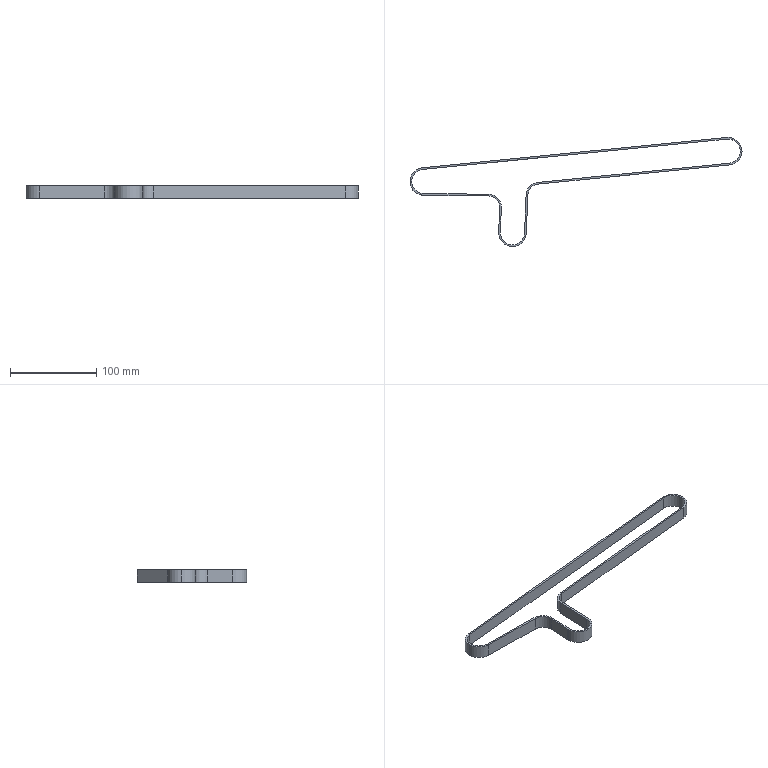Part | STEP file | HTBN918S3M-150 | 1 solid | 26 faces | box 383.9 x 126.27 x 15 mm | volume 27185 mm3 | cylinder 14 | plane 12 | commonest cylinder face diameters 27.9 x5 31.9 x5 25.8 x2 29.8 x2
STEP:
#1=CARTESIAN_POINT('',(-216.674,53.918,15.));
#2=VERTEX_POINT('',#1);
#3=CARTESIAN_POINT('',(-229.244,40.037,15.));
#4=VERTEX_POINT('',#3);
#5=CARTESIAN_POINT('',(-215.294,40.037,15.));
#6=DIRECTION('',(0.,0.,1.));
#7=DIRECTION('',(1.,0.,0.));
#8=AXIS2_PLACEMENT_3D('',#5,#6,#7);
#9=CIRCLE('',#8,13.95);
#10=EDGE_CURVE('',#2,#4,#9,.T.);
#11=ORIENTED_EDGE('',*,*,#10,.T.);
#12=CARTESIAN_POINT('',(-229.244,40.037,0.));
#13=VERTEX_POINT('',#12);
#14=CARTESIAN_POINT('',(-229.244,40.037,15.));
#15=DIRECTION('',(0.,0.,-1.));
#16=VECTOR('',#15,1000.);
#17=LINE('',#14,#16);
#18=EDGE_CURVE('',#4,#13,#17,.T.);
#19=ORIENTED_EDGE('',*,*,#18,.T.);
#20=CARTESIAN_POINT('',(-216.674,53.918,0.));
#21=VERTEX_POINT('',#20);
#22=CARTESIAN_POINT('',(-215.294,40.037,0.));
#23=DIRECTION('',(0.,0.,1.));
#24=DIRECTION('',(1.,0.,0.));
#25=AXIS2_PLACEMENT_3D('',#22,#23,#24);
#26=CIRCLE('',#25,13.95);
#27=EDGE_CURVE('',#21,#13,#26,.T.);
#28=ORIENTED_EDGE('',*,*,#27,.F.);
#29=CARTESIAN_POINT('',(-216.674,53.918,15.));
#30=DIRECTION('',(0.,0.,-1.));
#31=VECTOR('',#30,1000.);
#32=LINE('',#29,#31);
#33=EDGE_CURVE('',#2,#21,#32,.T.);
#34=ORIENTED_EDGE('',*,*,#33,.F.);
#35=EDGE_LOOP('',(#11,#19,#28,#34));
#36=FACE_OUTER_BOUND('',#35,.T.);
#37=CARTESIAN_POINT('',(-215.294,40.037,15.));
#38=DIRECTION('',(0.,0.,-1.));
#39=DIRECTION('',(-1.,0.,0.));
#40=AXIS2_PLACEMENT_3D('',#37,#38,#39);
#41=CYLINDRICAL_SURFACE('',#40,13.95);
#42=ADVANCED_FACE('',(#36),#41,.F.);
#43=CARTESIAN_POINT('',(-126.687,-18.819,15.));
#44=VERTEX_POINT('',#43);
#45=CARTESIAN_POINT('',(-126.697,-19.333,15.));
#46=VERTEX_POINT('',#45);
#47=CARTESIAN_POINT('',(-112.747,-19.333,15.));
#48=DIRECTION('',(0.,0.,1.));
#49=DIRECTION('',(1.,0.,0.));
#50=AXIS2_PLACEMENT_3D('',#47,#48,#49);
#51=CIRCLE('',#50,13.95);
#52=EDGE_CURVE('',#44,#46,#51,.T.);
#53=ORIENTED_EDGE('',*,*,#52,.T.);
#54=CARTESIAN_POINT('',(-126.697,-19.333,0.));
#55=VERTEX_POINT('',#54);
#56=CARTESIAN_POINT('',(-126.697,-19.333,15.));
#57=DIRECTION('',(0.,0.,-1.));
#58=VECTOR('',#57,1000.);
#59=LINE('',#56,#58);
#60=EDGE_CURVE('',#46,#55,#59,.T.);
#61=ORIENTED_EDGE('',*,*,#60,.T.);
#62=CARTESIAN_POINT('',(-126.687,-18.819,0.));
#63=VERTEX_POINT('',#62);
#64=CARTESIAN_POINT('',(-112.747,-19.333,0.));
#65=DIRECTION('',(0.,0.,1.));
#66=DIRECTION('',(1.,0.,0.));
#67=AXIS2_PLACEMENT_3D('',#64,#65,#66);
#68=CIRCLE('',#67,13.95);
#69=EDGE_CURVE('',#63,#55,#68,.T.);
#70=ORIENTED_EDGE('',*,*,#69,.F.);
#71=CARTESIAN_POINT('',(-126.687,-18.819,15.));
#72=DIRECTION('',(0.,0.,-1.));
#73=VECTOR('',#72,1000.);
#74=LINE('',#71,#73);
#75=EDGE_CURVE('',#44,#63,#74,.T.);
#76=ORIENTED_EDGE('',*,*,#75,.F.);
#77=EDGE_LOOP('',(#53,#61,#70,#76));
#78=FACE_OUTER_BOUND('',#77,.T.);
#79=CARTESIAN_POINT('',(-112.747,-19.333,15.));
#80=DIRECTION('',(0.,0.,-1.));
#81=DIRECTION('',(-1.,0.,0.));
#82=AXIS2_PLACEMENT_3D('',#79,#80,#81);
#83=CYLINDRICAL_SURFACE('',#82,13.95);
#84=ADVANCED_FACE('',(#78),#83,.F.);
#85=CARTESIAN_POINT('',(-128.697,-19.333,15.));
#86=VERTEX_POINT('',#85);
#87=CARTESIAN_POINT('',(-96.81,-19.979,15.));
#88=VERTEX_POINT('',#87);
#89=CARTESIAN_POINT('',(-112.747,-19.333,15.));
#90=DIRECTION('',(0.,0.,1.));
#91=DIRECTION('',(1.,0.,0.));
#92=AXIS2_PLACEMENT_3D('',#89,#90,#91);
#93=CIRCLE('',#92,15.95);
#94=EDGE_CURVE('',#86,#88,#93,.T.);
#95=ORIENTED_EDGE('',*,*,#94,.F.);
#96=CARTESIAN_POINT('',(-128.697,-19.333,0.));
#97=VERTEX_POINT('',#96);
#98=CARTESIAN_POINT('',(-128.697,-19.333,15.));
#99=DIRECTION('',(0.,0.,-1.));
#100=VECTOR('',#99,1000.);
#101=LINE('',#98,#100);
#102=EDGE_CURVE('',#86,#97,#101,.T.);
#103=ORIENTED_EDGE('',*,*,#102,.T.);
#104=CARTESIAN_POINT('',(-96.81,-19.979,0.));
#105=VERTEX_POINT('',#104);
#106=CARTESIAN_POINT('',(-112.747,-19.333,0.));
#107=DIRECTION('',(0.,0.,1.));
#108=DIRECTION('',(1.,0.,0.));
#109=AXIS2_PLACEMENT_3D('',#106,#107,#108);
#110=CIRCLE('',#109,15.95);
#111=EDGE_CURVE('',#97,#105,#110,.T.);
#112=ORIENTED_EDGE('',*,*,#111,.T.);
#113=CARTESIAN_POINT('',(-96.81,-19.979,15.));
#114=DIRECTION('',(0.,0.,-1.));
#115=VECTOR('',#114,1000.);
#116=LINE('',#113,#115);
#117=EDGE_CURVE('',#88,#105,#116,.T.);
#118=ORIENTED_EDGE('',*,*,#117,.F.);
#119=EDGE_LOOP('',(#95,#103,#112,#118));
#120=FACE_OUTER_BOUND('',#119,.T.);
#121=CARTESIAN_POINT('',(-112.747,-19.333,15.));
#122=DIRECTION('',(0.,0.,-1.));
#123=DIRECTION('',(-1.,0.,0.));
#124=AXIS2_PLACEMENT_3D('',#121,#122,#123);
#125=CYLINDRICAL_SURFACE('',#124,15.95);
#126=ADVANCED_FACE('',(#120),#125,.T.);
#127=CARTESIAN_POINT('',(-231.244,40.037,15.));
#128=VERTEX_POINT('',#127);
#129=CARTESIAN_POINT('',(-215.472,24.088,15.));
#130=VERTEX_POINT('',#129);
#131=CARTESIAN_POINT('',(-215.294,40.037,15.));
#132=DIRECTION('',(0.,0.,1.));
#133=DIRECTION('',(1.,0.,0.));
#134=AXIS2_PLACEMENT_3D('',#131,#132,#133);
#135=CIRCLE('',#134,15.95);
#136=EDGE_CURVE('',#128,#130,#135,.T.);
#137=ORIENTED_EDGE('',*,*,#136,.F.);
#138=CARTESIAN_POINT('',(-231.244,40.037,0.));
#139=VERTEX_POINT('',#138);
#140=CARTESIAN_POINT('',(-231.244,40.037,15.));
#141=DIRECTION('',(0.,0.,-1.));
#142=VECTOR('',#141,1000.);
#143=LINE('',#140,#142);
#144=EDGE_CURVE('',#128,#139,#143,.T.);
#145=ORIENTED_EDGE('',*,*,#144,.T.);
#146=CARTESIAN_POINT('',(-215.472,24.088,0.));
#147=VERTEX_POINT('',#146);
#148=CARTESIAN_POINT('',(-215.294,40.037,0.));
#149=DIRECTION('',(0.,0.,1.));
#150=DIRECTION('',(1.,0.,0.));
#151=AXIS2_PLACEMENT_3D('',#148,#149,#150);
#152=CIRCLE('',#151,15.95);
#153=EDGE_CURVE('',#139,#147,#152,.T.);
#154=ORIENTED_EDGE('',*,*,#153,.T.);
#155=CARTESIAN_POINT('',(-215.472,24.088,15.));
#156=DIRECTION('',(0.,0.,-1.));
#157=VECTOR('',#156,1000.);
#158=LINE('',#155,#157);
#159=EDGE_CURVE('',#130,#147,#158,.T.);
#160=ORIENTED_EDGE('',*,*,#159,.F.);
#161=EDGE_LOOP('',(#137,#145,#154,#160));
#162=FACE_OUTER_BOUND('',#161,.T.);
#163=CARTESIAN_POINT('',(-215.294,40.037,15.));
#164=DIRECTION('',(0.,0.,-1.));
#165=DIRECTION('',(-1.,0.,0.));
#166=AXIS2_PLACEMENT_3D('',#163,#164,#165);
#167=CYLINDRICAL_SURFACE('',#166,15.95);
#168=ADVANCED_FACE('',(#162),#167,.T.);
#169=CARTESIAN_POINT('',(-216.872,55.909,15.));
#170=VERTEX_POINT('',#169);
#171=CARTESIAN_POINT('',(-215.294,40.037,15.));
#172=DIRECTION('',(0.,0.,1.));
#173=DIRECTION('',(1.,0.,0.));
#174=AXIS2_PLACEMENT_3D('',#171,#172,#173);
#175=CIRCLE('',#174,15.95);
#176=EDGE_CURVE('',#170,#128,#175,.T.);
#177=ORIENTED_EDGE('',*,*,#176,.T.);
#178=ORIENTED_EDGE('',*,*,#136,.T.);
#179=CARTESIAN_POINT('',(-140.379,23.251,15.));
#180=VERTEX_POINT('',#179);
#181=CARTESIAN_POINT('',(-215.472,24.088,15.));
#182=DIRECTION('',(0.9999,-0.01115,0.));
#183=VECTOR('',#182,1000.);
#184=LINE('',#181,#183);
#185=EDGE_CURVE('',#130,#180,#184,.T.);
#186=ORIENTED_EDGE('',*,*,#185,.T.);
#187=CARTESIAN_POINT('',(-127.631,9.876,15.));
#188=VERTEX_POINT('',#187);
#189=CARTESIAN_POINT('',(-140.522,10.351,15.));
#190=DIRECTION('',(0.,0.,-1.));
#191=DIRECTION('',(1.,0.,0.));
#192=AXIS2_PLACEMENT_3D('',#189,#190,#191);
#193=CIRCLE('',#192,12.9);
#194=EDGE_CURVE('',#180,#188,#193,.T.);
#195=ORIENTED_EDGE('',*,*,#194,.T.);
#196=CARTESIAN_POINT('',(-128.686,-18.745,15.));
#197=VERTEX_POINT('',#196);
#198=CARTESIAN_POINT('',(-127.631,9.876,15.));
#199=DIRECTION('',(-0.03683,-0.9993,0.));
#200=VECTOR('',#199,1000.);
#201=LINE('',#198,#200);
#202=EDGE_CURVE('',#188,#197,#201,.T.);
#203=ORIENTED_EDGE('',*,*,#202,.T.);
#204=CARTESIAN_POINT('',(-112.747,-19.333,15.));
#205=DIRECTION('',(0.,0.,1.));
#206=DIRECTION('',(1.,0.,0.));
#207=AXIS2_PLACEMENT_3D('',#204,#205,#206);
#208=CIRCLE('',#207,15.95);
#209=EDGE_CURVE('',#197,#86,#208,.T.);
#210=ORIENTED_EDGE('',*,*,#209,.T.);
#211=ORIENTED_EDGE('',*,*,#94,.T.);
#212=CARTESIAN_POINT('',(-95.002,24.597,15.));
#213=VERTEX_POINT('',#212);
#214=CARTESIAN_POINT('',(-95.002,24.597,15.));
#215=DIRECTION('',(0.04052,0.9992,0.));
#216=VECTOR('',#215,1000.);
#217=LINE('',#214,#216);
#218=EDGE_CURVE('',#88,#213,#217,.T.);
#219=ORIENTED_EDGE('',*,*,#218,.T.);
#220=CARTESIAN_POINT('',(-83.401,36.91,15.));
#221=VERTEX_POINT('',#220);
#222=CARTESIAN_POINT('',(-82.113,24.074,15.));
#223=DIRECTION('',(0.,0.,-1.));
#224=DIRECTION('',(1.,0.,0.));
#225=AXIS2_PLACEMENT_3D('',#222,#223,#224);
#226=CIRCLE('',#225,12.9);
#227=EDGE_CURVE('',#213,#221,#226,.T.);
#228=ORIENTED_EDGE('',*,*,#227,.T.);
#229=CARTESIAN_POINT('',(138.299,59.167,15.));
#230=VERTEX_POINT('',#229);
#231=CARTESIAN_POINT('',(-83.401,36.91,15.));
#232=DIRECTION('',(0.995,0.09989,0.));
#233=VECTOR('',#232,1000.);
#234=LINE('',#231,#233);
#235=EDGE_CURVE('',#221,#230,#234,.T.);
#236=ORIENTED_EDGE('',*,*,#235,.T.);
#237=CARTESIAN_POINT('',(135.128,90.909,15.));
#238=VERTEX_POINT('',#237);
#239=CARTESIAN_POINT('',(136.706,75.037,15.));
#240=DIRECTION('',(0.,0.,1.));
#241=DIRECTION('',(1.,0.,0.));
#242=AXIS2_PLACEMENT_3D('',#239,#240,#241);
#243=CIRCLE('',#242,15.95);
#244=EDGE_CURVE('',#230,#238,#243,.T.);
#245=ORIENTED_EDGE('',*,*,#244,.T.);
#246=CARTESIAN_POINT('',(-216.872,55.909,15.));
#247=DIRECTION('',(-0.9951,-0.09894,0.));
#248=VECTOR('',#247,1000.);
#249=LINE('',#246,#248);
#250=EDGE_CURVE('',#238,#170,#249,.T.);
#251=ORIENTED_EDGE('',*,*,#250,.T.);
#252=EDGE_LOOP('',(#177,#178,#186,#195,#203,#210,#211,#219,#228,#236,#245,#251));
#253=FACE_OUTER_BOUND('',#252,.T.);
#254=CARTESIAN_POINT('',(-125.633,9.803,15.));
#255=VERTEX_POINT('',#254);
#256=CARTESIAN_POINT('',(-125.633,9.803,15.));
#257=DIRECTION('',(-0.03683,-0.9993,0.));
#258=VECTOR('',#257,1000.);
#259=LINE('',#256,#258);
#260=EDGE_CURVE('',#255,#44,#259,.T.);
#261=ORIENTED_EDGE('',*,*,#260,.F.);
#262=CARTESIAN_POINT('',(-140.356,25.25,15.));
#263=VERTEX_POINT('',#262);
#264=CARTESIAN_POINT('',(-140.522,10.351,15.));
#265=DIRECTION('',(0.,0.,-1.));
#266=DIRECTION('',(1.,0.,0.));
#267=AXIS2_PLACEMENT_3D('',#264,#265,#266);
#268=CIRCLE('',#267,14.9);
#269=EDGE_CURVE('',#263,#255,#268,.T.);
#270=ORIENTED_EDGE('',*,*,#269,.F.);
#271=CARTESIAN_POINT('',(-215.449,26.088,15.));
#272=VERTEX_POINT('',#271);
#273=CARTESIAN_POINT('',(-215.449,26.088,15.));
#274=DIRECTION('',(0.9999,-0.01115,0.));
#275=VECTOR('',#274,1000.);
#276=LINE('',#273,#275);
#277=EDGE_CURVE('',#272,#263,#276,.T.);
#278=ORIENTED_EDGE('',*,*,#277,.F.);
#279=CARTESIAN_POINT('',(-215.294,40.037,15.));
#280=DIRECTION('',(0.,0.,1.));
#281=DIRECTION('',(1.,0.,0.));
#282=AXIS2_PLACEMENT_3D('',#279,#280,#281);
#283=CIRCLE('',#282,13.95);
#284=EDGE_CURVE('',#4,#272,#283,.T.);
#285=ORIENTED_EDGE('',*,*,#284,.F.);
#286=ORIENTED_EDGE('',*,*,#10,.F.);
#287=CARTESIAN_POINT('',(135.326,88.918,15.));
#288=VERTEX_POINT('',#287);
#289=CARTESIAN_POINT('',(-216.674,53.918,15.));
#290=DIRECTION('',(-0.9951,-0.09894,0.));
#291=VECTOR('',#290,1000.);
#292=LINE('',#289,#291);
#293=EDGE_CURVE('',#288,#2,#292,.T.);
#294=ORIENTED_EDGE('',*,*,#293,.F.);
#295=CARTESIAN_POINT('',(138.1,61.157,15.));
#296=VERTEX_POINT('',#295);
#297=CARTESIAN_POINT('',(136.706,75.037,15.));
#298=DIRECTION('',(0.,0.,1.));
#299=DIRECTION('',(1.,0.,0.));
#300=AXIS2_PLACEMENT_3D('',#297,#298,#299);
#301=CIRCLE('',#300,13.95);
#302=EDGE_CURVE('',#296,#288,#301,.T.);
#303=ORIENTED_EDGE('',*,*,#302,.F.);
#304=CARTESIAN_POINT('',(-83.601,38.9,15.));
#305=VERTEX_POINT('',#304);
#306=CARTESIAN_POINT('',(-83.601,38.9,15.));
#307=DIRECTION('',(0.995,0.09989,0.));
#308=VECTOR('',#307,1000.);
#309=LINE('',#306,#308);
#310=EDGE_CURVE('',#305,#296,#309,.T.);
#311=ORIENTED_EDGE('',*,*,#310,.F.);
#312=CARTESIAN_POINT('',(-97.001,24.678,15.));
#313=VERTEX_POINT('',#312);
#314=CARTESIAN_POINT('',(-82.113,24.074,15.));
#315=DIRECTION('',(0.,0.,-1.));
#316=DIRECTION('',(1.,0.,0.));
#317=AXIS2_PLACEMENT_3D('',#314,#315,#316);
#318=CIRCLE('',#317,14.9);
#319=EDGE_CURVE('',#313,#305,#318,.T.);
#320=ORIENTED_EDGE('',*,*,#319,.F.);
#321=CARTESIAN_POINT('',(-98.808,-19.898,15.));
#322=VERTEX_POINT('',#321);
#323=CARTESIAN_POINT('',(-97.001,24.678,15.));
#324=DIRECTION('',(0.04052,0.9992,0.));
#325=VECTOR('',#324,1000.);
#326=LINE('',#323,#325);
#327=EDGE_CURVE('',#322,#313,#326,.T.);
#328=ORIENTED_EDGE('',*,*,#327,.F.);
#329=CARTESIAN_POINT('',(-112.747,-19.333,15.));
#330=DIRECTION('',(0.,0.,1.));
#331=DIRECTION('',(1.,0.,0.));
#332=AXIS2_PLACEMENT_3D('',#329,#330,#331);
#333=CIRCLE('',#332,13.95);
#334=EDGE_CURVE('',#46,#322,#333,.T.);
#335=ORIENTED_EDGE('',*,*,#334,.F.);
#336=ORIENTED_EDGE('',*,*,#52,.F.);
#337=EDGE_LOOP('',(#261,#270,#278,#285,#286,#294,#303,#311,#320,#328,#335,#336));
#338=FACE_BOUND('',#337,.T.);
#339=CARTESIAN_POINT('',(-215.294,40.037,15.));
#340=DIRECTION('',(0.,0.,1.));
#341=DIRECTION('',(1.,0.,0.));
#342=AXIS2_PLACEMENT_3D('',#339,#340,#341);
#343=PLANE('',#342);
#344=ADVANCED_FACE('',(#253,#338),#343,.T.);
#345=CARTESIAN_POINT('',(-216.872,55.909,0.));
#346=VERTEX_POINT('',#345);
#347=CARTESIAN_POINT('',(-215.294,40.037,0.));
#348=DIRECTION('',(0.,0.,1.));
#349=DIRECTION('',(1.,0.,0.));
#350=AXIS2_PLACEMENT_3D('',#347,#348,#349);
#351=CIRCLE('',#350,15.95);
#352=EDGE_CURVE('',#346,#139,#351,.T.);
#353=ORIENTED_EDGE('',*,*,#352,.F.);
#354=CARTESIAN_POINT('',(135.128,90.909,0.));
#355=VERTEX_POINT('',#354);
#356=CARTESIAN_POINT('',(-216.872,55.909,0.));
#357=DIRECTION('',(-0.9951,-0.09894,0.));
#358=VECTOR('',#357,1000.);
#359=LINE('',#356,#358);
#360=EDGE_CURVE('',#355,#346,#359,.T.);
#361=ORIENTED_EDGE('',*,*,#360,.F.);
#362=CARTESIAN_POINT('',(138.299,59.167,0.));
#363=VERTEX_POINT('',#362);
#364=CARTESIAN_POINT('',(136.706,75.037,0.));
#365=DIRECTION('',(0.,0.,1.));
#366=DIRECTION('',(1.,0.,0.));
#367=AXIS2_PLACEMENT_3D('',#364,#365,#366);
#368=CIRCLE('',#367,15.95);
#369=EDGE_CURVE('',#363,#355,#368,.T.);
#370=ORIENTED_EDGE('',*,*,#369,.F.);
#371=CARTESIAN_POINT('',(-83.401,36.91,0.));
#372=VERTEX_POINT('',#371);
#373=CARTESIAN_POINT('',(-83.401,36.91,0.));
#374=DIRECTION('',(0.995,0.09989,0.));
#375=VECTOR('',#374,1000.);
#376=LINE('',#373,#375);
#377=EDGE_CURVE('',#372,#363,#376,.T.);
#378=ORIENTED_EDGE('',*,*,#377,.F.);
#379=CARTESIAN_POINT('',(-95.002,24.597,0.));
#380=VERTEX_POINT('',#379);
#381=CARTESIAN_POINT('',(-82.113,24.074,0.));
#382=DIRECTION('',(0.,0.,-1.));
#383=DIRECTION('',(1.,0.,0.));
#384=AXIS2_PLACEMENT_3D('',#381,#382,#383);
#385=CIRCLE('',#384,12.9);
#386=EDGE_CURVE('',#380,#372,#385,.T.);
#387=ORIENTED_EDGE('',*,*,#386,.F.);
#388=CARTESIAN_POINT('',(-95.002,24.597,0.));
#389=DIRECTION('',(0.04052,0.9992,0.));
#390=VECTOR('',#389,1000.);
#391=LINE('',#388,#390);
#392=EDGE_CURVE('',#105,#380,#391,.T.);
#393=ORIENTED_EDGE('',*,*,#392,.F.);
#394=ORIENTED_EDGE('',*,*,#111,.F.);
#395=CARTESIAN_POINT('',(-128.686,-18.745,0.));
#396=VERTEX_POINT('',#395);
#397=CARTESIAN_POINT('',(-112.747,-19.333,0.));
#398=DIRECTION('',(0.,0.,1.));
#399=DIRECTION('',(1.,0.,0.));
#400=AXIS2_PLACEMENT_3D('',#397,#398,#399);
#401=CIRCLE('',#400,15.95);
#402=EDGE_CURVE('',#396,#97,#401,.T.);
#403=ORIENTED_EDGE('',*,*,#402,.F.);
#404=CARTESIAN_POINT('',(-127.631,9.876,0.));
#405=VERTEX_POINT('',#404);
#406=CARTESIAN_POINT('',(-127.631,9.876,0.));
#407=DIRECTION('',(-0.03683,-0.9993,0.));
#408=VECTOR('',#407,1000.);
#409=LINE('',#406,#408);
#410=EDGE_CURVE('',#405,#396,#409,.T.);
#411=ORIENTED_EDGE('',*,*,#410,.F.);
#412=CARTESIAN_POINT('',(-140.379,23.251,0.));
#413=VERTEX_POINT('',#412);
#414=CARTESIAN_POINT('',(-140.522,10.351,0.));
#415=DIRECTION('',(0.,0.,-1.));
#416=DIRECTION('',(1.,0.,0.));
#417=AXIS2_PLACEMENT_3D('',#414,#415,#416);
#418=CIRCLE('',#417,12.9);
#419=EDGE_CURVE('',#413,#405,#418,.T.);
#420=ORIENTED_EDGE('',*,*,#419,.F.);
#421=CARTESIAN_POINT('',(-215.472,24.088,0.));
#422=DIRECTION('',(0.9999,-0.01115,0.));
#423=VECTOR('',#422,1000.);
#424=LINE('',#421,#423);
#425=EDGE_CURVE('',#147,#413,#424,.T.);
#426=ORIENTED_EDGE('',*,*,#425,.F.);
#427=ORIENTED_EDGE('',*,*,#153,.F.);
#428=EDGE_LOOP('',(#353,#361,#370,#378,#387,#393,#394,#403,#411,#420,#426,#427));
#429=FACE_OUTER_BOUND('',#428,.T.);
#430=CARTESIAN_POINT('',(-140.356,25.25,0.));
#431=VERTEX_POINT('',#430);
#432=CARTESIAN_POINT('',(-125.633,9.803,0.));
#433=VERTEX_POINT('',#432);
#434=CARTESIAN_POINT('',(-140.522,10.351,0.));
#435=DIRECTION('',(0.,0.,-1.));
#436=DIRECTION('',(1.,0.,0.));
#437=AXIS2_PLACEMENT_3D('',#434,#435,#436);
#438=CIRCLE('',#437,14.9);
#439=EDGE_CURVE('',#431,#433,#438,.T.);
#440=ORIENTED_EDGE('',*,*,#439,.T.);
#441=CARTESIAN_POINT('',(-125.633,9.803,0.));
#442=DIRECTION('',(-0.03683,-0.9993,0.));
#443=VECTOR('',#442,1000.);
#444=LINE('',#441,#443);
#445=EDGE_CURVE('',#433,#63,#444,.T.);
#446=ORIENTED_EDGE('',*,*,#445,.T.);
#447=ORIENTED_EDGE('',*,*,#69,.T.);
#448=CARTESIAN_POINT('',(-98.808,-19.898,0.));
#449=VERTEX_POINT('',#448);
#450=CARTESIAN_POINT('',(-112.747,-19.333,0.));
#451=DIRECTION('',(0.,0.,1.));
#452=DIRECTION('',(1.,0.,0.));
#453=AXIS2_PLACEMENT_3D('',#450,#451,#452);
#454=CIRCLE('',#453,13.95);
#455=EDGE_CURVE('',#55,#449,#454,.T.);
#456=ORIENTED_EDGE('',*,*,#455,.T.);
#457=CARTESIAN_POINT('',(-97.001,24.678,0.));
#458=VERTEX_POINT('',#457);
#459=CARTESIAN_POINT('',(-97.001,24.678,0.));
#460=DIRECTION('',(0.04052,0.9992,0.));
#461=VECTOR('',#460,1000.);
#462=LINE('',#459,#461);
#463=EDGE_CURVE('',#449,#458,#462,.T.);
#464=ORIENTED_EDGE('',*,*,#463,.T.);
#465=CARTESIAN_POINT('',(-83.601,38.9,0.));
#466=VERTEX_POINT('',#465);
#467=CARTESIAN_POINT('',(-82.113,24.074,0.));
#468=DIRECTION('',(0.,0.,-1.));
#469=DIRECTION('',(1.,0.,0.));
#470=AXIS2_PLACEMENT_3D('',#467,#468,#469);
#471=CIRCLE('',#470,14.9);
#472=EDGE_CURVE('',#458,#466,#471,.T.);
#473=ORIENTED_EDGE('',*,*,#472,.T.);
#474=CARTESIAN_POINT('',(138.1,61.157,0.));
#475=VERTEX_POINT('',#474);
#476=CARTESIAN_POINT('',(-83.601,38.9,0.));
#477=DIRECTION('',(0.995,0.09989,0.));
#478=VECTOR('',#477,1000.);
#479=LINE('',#476,#478);
#480=EDGE_CURVE('',#466,#475,#479,.T.);
#481=ORIENTED_EDGE('',*,*,#480,.T.);
#482=CARTESIAN_POINT('',(135.326,88.918,0.));
#483=VERTEX_POINT('',#482);
#484=CARTESIAN_POINT('',(136.706,75.037,0.));
#485=DIRECTION('',(0.,0.,1.));
#486=DIRECTION('',(1.,0.,0.));
#487=AXIS2_PLACEMENT_3D('',#484,#485,#486);
#488=CIRCLE('',#487,13.95);
#489=EDGE_CURVE('',#475,#483,#488,.T.);
#490=ORIENTED_EDGE('',*,*,#489,.T.);
#491=CARTESIAN_POINT('',(-216.674,53.918,0.));
#492=DIRECTION('',(-0.9951,-0.09894,0.));
#493=VECTOR('',#492,1000.);
#494=LINE('',#491,#493);
#495=EDGE_CURVE('',#483,#21,#494,.T.);
#496=ORIENTED_EDGE('',*,*,#495,.T.);
#497=ORIENTED_EDGE('',*,*,#27,.T.);
#498=CARTESIAN_POINT('',(-215.449,26.088,0.));
#499=VERTEX_POINT('',#498);
#500=CARTESIAN_POINT('',(-215.294,40.037,0.));
#501=DIRECTION('',(0.,0.,1.));
#502=DIRECTION('',(1.,0.,0.));
#503=AXIS2_PLACEMENT_3D('',#500,#501,#502);
#504=CIRCLE('',#503,13.95);
#505=EDGE_CURVE('',#13,#499,#504,.T.);
#506=ORIENTED_EDGE('',*,*,#505,.T.);
#507=CARTESIAN_POINT('',(-215.449,26.088,0.));
#508=DIRECTION('',(0.9999,-0.01115,0.));
#509=VECTOR('',#508,1000.);
#510=LINE('',#507,#509);
#511=EDGE_CURVE('',#499,#431,#510,.T.);
#512=ORIENTED_EDGE('',*,*,#511,.T.);
#513=EDGE_LOOP('',(#440,#446,#447,#456,#464,#473,#481,#490,#496,#497,#506,#512));
#514=FACE_BOUND('',#513,.T.);
#515=CARTESIAN_POINT('',(-215.294,40.037,0.));
#516=DIRECTION('',(0.,0.,1.));
#517=DIRECTION('',(1.,0.,0.));
#518=AXIS2_PLACEMENT_3D('',#515,#516,#517);
#519=PLANE('',#518);
#520=ADVANCED_FACE('',(#429,#514),#519,.F.);
#521=ORIENTED_EDGE('',*,*,#144,.F.);
#522=ORIENTED_EDGE('',*,*,#176,.F.);
#523=CARTESIAN_POINT('',(-216.872,55.909,15.));
#524=DIRECTION('',(0.,0.,-1.));
#525=VECTOR('',#524,1000.);
#526=LINE('',#523,#525);
#527=EDGE_CURVE('',#170,#346,#526,.T.);
#528=ORIENTED_EDGE('',*,*,#527,.T.);
#529=ORIENTED_EDGE('',*,*,#352,.T.);
#530=EDGE_LOOP('',(#521,#522,#528,#529));
#531=FACE_OUTER_BOUND('',#530,.T.);
#532=CARTESIAN_POINT('',(-215.294,40.037,15.));
#533=DIRECTION('',(0.,0.,-1.));
#534=DIRECTION('',(-1.,0.,0.));
#535=AXIS2_PLACEMENT_3D('',#532,#533,#534);
#536=CYLINDRICAL_SURFACE('',#535,15.95);
#537=ADVANCED_FACE('',(#531),#536,.T.);
#538=ORIENTED_EDGE('',*,*,#425,.T.);
#539=CARTESIAN_POINT('',(-140.379,23.251,15.));
#540=DIRECTION('',(0.,0.,-1.));
#541=VECTOR('',#540,1000.);
#542=LINE('',#539,#541);
#543=EDGE_CURVE('',#180,#413,#542,.T.);
#544=ORIENTED_EDGE('',*,*,#543,.F.);
#545=ORIENTED_EDGE('',*,*,#185,.F.);
#546=ORIENTED_EDGE('',*,*,#159,.T.);
#547=EDGE_LOOP('',(#538,#544,#545,#546));
#548=FACE_OUTER_BOUND('',#547,.T.);
#549=CARTESIAN_POINT('',(-215.472,24.088,15.));
#550=DIRECTION('',(0.01115,0.9999,0.));
#551=DIRECTION('',(-0.9999,0.01115,0.));
#552=AXIS2_PLACEMENT_3D('',#549,#550,#551);
#553=PLANE('',#552);
#554=ADVANCED_FACE('',(#548),#553,.F.);
#555=ORIENTED_EDGE('',*,*,#419,.T.);
#556=CARTESIAN_POINT('',(-127.631,9.876,15.));
#557=DIRECTION('',(0.,0.,-1.));
#558=VECTOR('',#557,1000.);
#559=LINE('',#556,#558);
#560=EDGE_CURVE('',#188,#405,#559,.T.);
#561=ORIENTED_EDGE('',*,*,#560,.F.);
#562=ORIENTED_EDGE('',*,*,#194,.F.);
#563=ORIENTED_EDGE('',*,*,#543,.T.);
#564=EDGE_LOOP('',(#555,#561,#562,#563));
#565=FACE_OUTER_BOUND('',#564,.T.);
#566=CARTESIAN_POINT('',(-140.522,10.351,15.));
#567=DIRECTION('',(0.,0.,-1.));
#568=DIRECTION('',(-1.,0.,0.));
#569=AXIS2_PLACEMENT_3D('',#566,#567,#568);
#570=CYLINDRICAL_SURFACE('',#569,12.9);
#571=ADVANCED_FACE('',(#565),#570,.F.);
#572=ORIENTED_EDGE('',*,*,#410,.T.);
#573=CARTESIAN_POINT('',(-128.686,-18.745,15.));
#574=DIRECTION('',(0.,0.,-1.));
#575=VECTOR('',#574,1000.);
#576=LINE('',#573,#575);
#577=EDGE_CURVE('',#197,#396,#576,.T.);
#578=ORIENTED_EDGE('',*,*,#577,.F.);
#579=ORIENTED_EDGE('',*,*,#202,.F.);
#580=ORIENTED_EDGE('',*,*,#560,.T.);
#581=EDGE_LOOP('',(#572,#578,#579,#580));
#582=FACE_OUTER_BOUND('',#581,.T.);
#583=CARTESIAN_POINT('',(-127.631,9.876,15.));
#584=DIRECTION('',(0.9993,-0.03683,0.));
#585=DIRECTION('',(0.03683,0.9993,0.));
#586=AXIS2_PLACEMENT_3D('',#583,#584,#585);
#587=PLANE('',#586);
#588=ADVANCED_FACE('',(#582),#587,.F.);
#589=ORIENTED_EDGE('',*,*,#102,.F.);
#590=ORIENTED_EDGE('',*,*,#209,.F.);
#591=ORIENTED_EDGE('',*,*,#577,.T.);
#592=ORIENTED_EDGE('',*,*,#402,.T.);
#593=EDGE_LOOP('',(#589,#590,#591,#592));
#594=FACE_OUTER_BOUND('',#593,.T.);
#595=CARTESIAN_POINT('',(-112.747,-19.333,15.));
#596=DIRECTION('',(0.,0.,-1.));
#597=DIRECTION('',(-1.,0.,0.));
#598=AXIS2_PLACEMENT_3D('',#595,#596,#597);
#599=CYLINDRICAL_SURFACE('',#598,15.95);
#600=ADVANCED_FACE('',(#594),#599,.T.);
#601=ORIENTED_EDGE('',*,*,#392,.T.);
#602=CARTESIAN_POINT('',(-95.002,24.597,15.));
#603=DIRECTION('',(0.,0.,-1.));
#604=VECTOR('',#603,1000.);
#605=LINE('',#602,#604);
#606=EDGE_CURVE('',#213,#380,#605,.T.);
#607=ORIENTED_EDGE('',*,*,#606,.F.);
#608=ORIENTED_EDGE('',*,*,#218,.F.);
#609=ORIENTED_EDGE('',*,*,#117,.T.);
#610=EDGE_LOOP('',(#601,#607,#608,#609));
#611=FACE_OUTER_BOUND('',#610,.T.);
#612=CARTESIAN_POINT('',(-95.002,24.597,15.));
#613=DIRECTION('',(-0.9992,0.04052,0.));
#614=DIRECTION('',(-0.04052,-0.9992,0.));
#615=AXIS2_PLACEMENT_3D('',#612,#613,#614);
#616=PLANE('',#615);
#617=ADVANCED_FACE('',(#611),#616,.F.);
#618=ORIENTED_EDGE('',*,*,#386,.T.);
#619=CARTESIAN_POINT('',(-83.401,36.91,15.));
#620=DIRECTION('',(0.,0.,-1.));
#621=VECTOR('',#620,1000.);
#622=LINE('',#619,#621);
#623=EDGE_CURVE('',#221,#372,#622,.T.);
#624=ORIENTED_EDGE('',*,*,#623,.F.);
#625=ORIENTED_EDGE('',*,*,#227,.F.);
#626=ORIENTED_EDGE('',*,*,#606,.T.);
#627=EDGE_LOOP('',(#618,#624,#625,#626));
#628=FACE_OUTER_BOUND('',#627,.T.);
#629=CARTESIAN_POINT('',(-82.113,24.074,15.));
#630=DIRECTION('',(0.,0.,-1.));
#631=DIRECTION('',(-1.,0.,0.));
#632=AXIS2_PLACEMENT_3D('',#629,#630,#631);
#633=CYLINDRICAL_SURFACE('',#632,12.9);
#634=ADVANCED_FACE('',(#628),#633,.F.);
#635=ORIENTED_EDGE('',*,*,#377,.T.);
#636=CARTESIAN_POINT('',(138.299,59.167,15.));
#637=DIRECTION('',(0.,0.,-1.));
#638=VECTOR('',#637,1000.);
#639=LINE('',#636,#638);
#640=EDGE_CURVE('',#230,#363,#639,.T.);
#641=ORIENTED_EDGE('',*,*,#640,.F.);
#642=ORIENTED_EDGE('',*,*,#235,.F.);
#643=ORIENTED_EDGE('',*,*,#623,.T.);
#644=EDGE_LOOP('',(#635,#641,#642,#643));
#645=FACE_OUTER_BOUND('',#644,.T.);
#646=CARTESIAN_POINT('',(-83.401,36.91,15.));
#647=DIRECTION('',(-0.09989,0.995,0.));
#648=DIRECTION('',(-0.995,-0.09989,0.));
#649=AXIS2_PLACEMENT_3D('',#646,#647,#648);
#650=PLANE('',#649);
#651=ADVANCED_FACE('',(#645),#650,.F.);
#652=ORIENTED_EDGE('',*,*,#369,.T.);
#653=CARTESIAN_POINT('',(135.128,90.909,15.));
#654=DIRECTION('',(0.,0.,-1.));
#655=VECTOR('',#654,1000.);
#656=LINE('',#653,#655);
#657=EDGE_CURVE('',#238,#355,#656,.T.);
#658=ORIENTED_EDGE('',*,*,#657,.F.);
#659=ORIENTED_EDGE('',*,*,#244,.F.);
#660=ORIENTED_EDGE('',*,*,#640,.T.);
#661=EDGE_LOOP('',(#652,#658,#659,#660));
#662=FACE_OUTER_BOUND('',#661,.T.);
#663=CARTESIAN_POINT('',(136.706,75.037,15.));
#664=DIRECTION('',(0.,0.,-1.));
#665=DIRECTION('',(-1.,0.,0.));
#666=AXIS2_PLACEMENT_3D('',#663,#664,#665);
#667=CYLINDRICAL_SURFACE('',#666,15.95);
#668=ADVANCED_FACE('',(#662),#667,.T.);
#669=ORIENTED_EDGE('',*,*,#360,.T.);
#670=ORIENTED_EDGE('',*,*,#527,.F.);
#671=ORIENTED_EDGE('',*,*,#250,.F.);
#672=ORIENTED_EDGE('',*,*,#657,.T.);
#673=EDGE_LOOP('',(#669,#670,#671,#672));
#674=FACE_OUTER_BOUND('',#673,.T.);
#675=CARTESIAN_POINT('',(-216.872,55.909,15.));
#676=DIRECTION('',(0.09894,-0.9951,0.));
#677=DIRECTION('',(0.9951,0.09894,0.));
#678=AXIS2_PLACEMENT_3D('',#675,#676,#677);
#679=PLANE('',#678);
#680=ADVANCED_FACE('',(#674),#679,.F.);
#681=ORIENTED_EDGE('',*,*,#439,.F.);
#682=CARTESIAN_POINT('',(-140.356,25.25,15.));
#683=DIRECTION('',(0.,0.,-1.));
#684=VECTOR('',#683,1000.);
#685=LINE('',#682,#684);
#686=EDGE_CURVE('',#263,#431,#685,.T.);
#687=ORIENTED_EDGE('',*,*,#686,.F.);
#688=ORIENTED_EDGE('',*,*,#269,.T.);
#689=CARTESIAN_POINT('',(-125.633,9.803,15.));
#690=DIRECTION('',(0.,0.,-1.));
#691=VECTOR('',#690,1000.);
#692=LINE('',#689,#691);
#693=EDGE_CURVE('',#255,#433,#692,.T.);
#694=ORIENTED_EDGE('',*,*,#693,.T.);
#695=EDGE_LOOP('',(#681,#687,#688,#694));
#696=FACE_OUTER_BOUND('',#695,.T.);
#697=CARTESIAN_POINT('',(-140.522,10.351,15.));
#698=DIRECTION('',(0.,0.,-1.));
#699=DIRECTION('',(-1.,0.,0.));
#700=AXIS2_PLACEMENT_3D('',#697,#698,#699);
#701=CYLINDRICAL_SURFACE('',#700,14.9);
#702=ADVANCED_FACE('',(#696),#701,.T.);
#703=ORIENTED_EDGE('',*,*,#445,.F.);
#704=ORIENTED_EDGE('',*,*,#693,.F.);
#705=ORIENTED_EDGE('',*,*,#260,.T.);
#706=ORIENTED_EDGE('',*,*,#75,.T.);
#707=EDGE_LOOP('',(#703,#704,#705,#706));
#708=FACE_OUTER_BOUND('',#707,.T.);
#709=CARTESIAN_POINT('',(-125.633,9.803,15.));
#710=DIRECTION('',(0.9993,-0.03683,0.));
#711=DIRECTION('',(0.03683,0.9993,0.));
#712=AXIS2_PLACEMENT_3D('',#709,#710,#711);
#713=PLANE('',#712);
#714=ADVANCED_FACE('',(#708),#713,.T.);
#715=ORIENTED_EDGE('',*,*,#60,.F.);
#716=ORIENTED_EDGE('',*,*,#334,.T.);
#717=CARTESIAN_POINT('',(-98.808,-19.898,15.));
#718=DIRECTION('',(0.,0.,-1.));
#719=VECTOR('',#718,1000.);
#720=LINE('',#717,#719);
#721=EDGE_CURVE('',#322,#449,#720,.T.);
#722=ORIENTED_EDGE('',*,*,#721,.T.);
#723=ORIENTED_EDGE('',*,*,#455,.F.);
#724=EDGE_LOOP('',(#715,#716,#722,#723));
#725=FACE_OUTER_BOUND('',#724,.T.);
#726=CARTESIAN_POINT('',(-112.747,-19.333,15.));
#727=DIRECTION('',(0.,0.,-1.));
#728=DIRECTION('',(-1.,0.,0.));
#729=AXIS2_PLACEMENT_3D('',#726,#727,#728);
#730=CYLINDRICAL_SURFACE('',#729,13.95);
#731=ADVANCED_FACE('',(#725),#730,.F.);
#732=ORIENTED_EDGE('',*,*,#463,.F.);
#733=ORIENTED_EDGE('',*,*,#721,.F.);
#734=ORIENTED_EDGE('',*,*,#327,.T.);
#735=CARTESIAN_POINT('',(-97.001,24.678,15.));
#736=DIRECTION('',(0.,0.,-1.));
#737=VECTOR('',#736,1000.);
#738=LINE('',#735,#737);
#739=EDGE_CURVE('',#313,#458,#738,.T.);
#740=ORIENTED_EDGE('',*,*,#739,.T.);
#741=EDGE_LOOP('',(#732,#733,#734,#740));
#742=FACE_OUTER_BOUND('',#741,.T.);
#743=CARTESIAN_POINT('',(-97.001,24.678,15.));
#744=DIRECTION('',(-0.9992,0.04052,0.));
#745=DIRECTION('',(-0.04052,-0.9992,0.));
#746=AXIS2_PLACEMENT_3D('',#743,#744,#745);
#747=PLANE('',#746);
#748=ADVANCED_FACE('',(#742),#747,.T.);
#749=ORIENTED_EDGE('',*,*,#472,.F.);
#750=ORIENTED_EDGE('',*,*,#739,.F.);
#751=ORIENTED_EDGE('',*,*,#319,.T.);
#752=CARTESIAN_POINT('',(-83.601,38.9,15.));
#753=DIRECTION('',(0.,0.,-1.));
#754=VECTOR('',#753,1000.);
#755=LINE('',#752,#754);
#756=EDGE_CURVE('',#305,#466,#755,.T.);
#757=ORIENTED_EDGE('',*,*,#756,.T.);
#758=EDGE_LOOP('',(#749,#750,#751,#757));
#759=FACE_OUTER_BOUND('',#758,.T.);
#760=CARTESIAN_POINT('',(-82.113,24.074,15.));
#761=DIRECTION('',(0.,0.,-1.));
#762=DIRECTION('',(-1.,0.,0.));
#763=AXIS2_PLACEMENT_3D('',#760,#761,#762);
#764=CYLINDRICAL_SURFACE('',#763,14.9);
#765=ADVANCED_FACE('',(#759),#764,.T.);
#766=ORIENTED_EDGE('',*,*,#480,.F.);
#767=ORIENTED_EDGE('',*,*,#756,.F.);
#768=ORIENTED_EDGE('',*,*,#310,.T.);
#769=CARTESIAN_POINT('',(138.1,61.157,15.));
#770=DIRECTION('',(0.,0.,-1.));
#771=VECTOR('',#770,1000.);
#772=LINE('',#769,#771);
#773=EDGE_CURVE('',#296,#475,#772,.T.);
#774=ORIENTED_EDGE('',*,*,#773,.T.);
#775=EDGE_LOOP('',(#766,#767,#768,#774));
#776=FACE_OUTER_BOUND('',#775,.T.);
#777=CARTESIAN_POINT('',(-83.601,38.9,15.));
#778=DIRECTION('',(-0.09989,0.995,0.));
#779=DIRECTION('',(-0.995,-0.09989,0.));
#780=AXIS2_PLACEMENT_3D('',#777,#778,#779);
#781=PLANE('',#780);
#782=ADVANCED_FACE('',(#776),#781,.T.);
#783=ORIENTED_EDGE('',*,*,#489,.F.);
#784=ORIENTED_EDGE('',*,*,#773,.F.);
#785=ORIENTED_EDGE('',*,*,#302,.T.);
#786=CARTESIAN_POINT('',(135.326,88.918,15.));
#787=DIRECTION('',(0.,0.,-1.));
#788=VECTOR('',#787,1000.);
#789=LINE('',#786,#788);
#790=EDGE_CURVE('',#288,#483,#789,.T.);
#791=ORIENTED_EDGE('',*,*,#790,.T.);
#792=EDGE_LOOP('',(#783,#784,#785,#791));
#793=FACE_OUTER_BOUND('',#792,.T.);
#794=CARTESIAN_POINT('',(136.706,75.037,15.));
#795=DIRECTION('',(0.,0.,-1.));
#796=DIRECTION('',(-1.,0.,0.));
#797=AXIS2_PLACEMENT_3D('',#794,#795,#796);
#798=CYLINDRICAL_SURFACE('',#797,13.95);
#799=ADVANCED_FACE('',(#793),#798,.F.);
#800=ORIENTED_EDGE('',*,*,#495,.F.);
#801=ORIENTED_EDGE('',*,*,#790,.F.);
#802=ORIENTED_EDGE('',*,*,#293,.T.);
#803=ORIENTED_EDGE('',*,*,#33,.T.);
#804=EDGE_LOOP('',(#800,#801,#802,#803));
#805=FACE_OUTER_BOUND('',#804,.T.);
#806=CARTESIAN_POINT('',(-216.674,53.918,15.));
#807=DIRECTION('',(0.09894,-0.9951,0.));
#808=DIRECTION('',(0.9951,0.09894,0.));
#809=AXIS2_PLACEMENT_3D('',#806,#807,#808);
#810=PLANE('',#809);
#811=ADVANCED_FACE('',(#805),#810,.T.);
#812=ORIENTED_EDGE('',*,*,#18,.F.);
#813=ORIENTED_EDGE('',*,*,#284,.T.);
#814=CARTESIAN_POINT('',(-215.449,26.088,15.));
#815=DIRECTION('',(0.,0.,-1.));
#816=VECTOR('',#815,1000.);
#817=LINE('',#814,#816);
#818=EDGE_CURVE('',#272,#499,#817,.T.);
#819=ORIENTED_EDGE('',*,*,#818,.T.);
#820=ORIENTED_EDGE('',*,*,#505,.F.);
#821=EDGE_LOOP('',(#812,#813,#819,#820));
#822=FACE_OUTER_BOUND('',#821,.T.);
#823=CARTESIAN_POINT('',(-215.294,40.037,15.));
#824=DIRECTION('',(0.,0.,-1.));
#825=DIRECTION('',(-1.,0.,0.));
#826=AXIS2_PLACEMENT_3D('',#823,#824,#825);
#827=CYLINDRICAL_SURFACE('',#826,13.95);
#828=ADVANCED_FACE('',(#822),#827,.F.);
#829=ORIENTED_EDGE('',*,*,#511,.F.);
#830=ORIENTED_EDGE('',*,*,#818,.F.);
#831=ORIENTED_EDGE('',*,*,#277,.T.);
#832=ORIENTED_EDGE('',*,*,#686,.T.);
#833=EDGE_LOOP('',(#829,#830,#831,#832));
#834=FACE_OUTER_BOUND('',#833,.T.);
#835=CARTESIAN_POINT('',(-215.449,26.088,15.));
#836=DIRECTION('',(0.01115,0.9999,0.));
#837=DIRECTION('',(-0.9999,0.01115,0.));
#838=AXIS2_PLACEMENT_3D('',#835,#836,#837);
#839=PLANE('',#838);
#840=ADVANCED_FACE('',(#834),#839,.T.);
#841=CLOSED_SHELL('',(#42,#84,#126,#168,#344,#520,#537,#554,#571,#588,#600,#617,#634,#651,#668,#680,#702,#714,#731,#748,#765,#782,#799,#811,#828,#840));
#842=MANIFOLD_SOLID_BREP('',#841);
#843=CARTESIAN_POINT('',(0.,0.,0.));
#844=DIRECTION('',(0.,0.,1.));
#845=DIRECTION('',(1.,0.,0.));
#846=AXIS2_PLACEMENT_3D('',#843,#844,#845);
#847=(LENGTH_UNIT()NAMED_UNIT(*)SI_UNIT(.MILLI.,.METRE.));
#848=UNCERTAINTY_MEASURE_WITH_UNIT(LENGTH_MEASURE(0.00001),#847,'','');
#849=(NAMED_UNIT(*)PLANE_ANGLE_UNIT()SI_UNIT($,.RADIAN.));
#850=(NAMED_UNIT(*)SI_UNIT($,.STERADIAN.)SOLID_ANGLE_UNIT());
#851=(GEOMETRIC_REPRESENTATION_CONTEXT(3)GLOBAL_UNCERTAINTY_ASSIGNED_CONTEXT((#848))GLOBAL_UNIT_ASSIGNED_CONTEXT((#847,#849,#850))REPRESENTATION_CONTEXT('',''));
#852=ADVANCED_BREP_SHAPE_REPRESENTATION('',(#842,#846),#851);